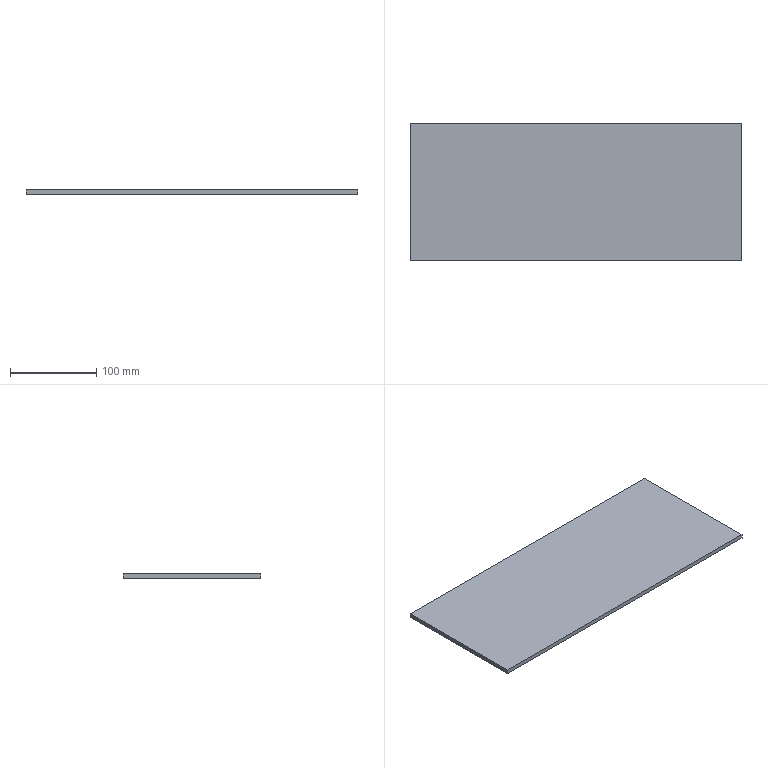Part | STEP file | FHD-021-014-03 acrylic | 1 solid | 6 faces | box 385 x 160 x 5 mm | volume 308000 mm3 | plane 6
STEP:
#1=CARTESIAN_POINT('',(0.,0.,0.));
#2=DIRECTION('',(0.,0.,1.));
#3=DIRECTION('',(1.,0.,0.));
#4=AXIS2_PLACEMENT_3D('',#1,#2,#3);
#5=CARTESIAN_POINT('',(-192.5,80.,5.));
#6=VERTEX_POINT('',#5);
#7=CARTESIAN_POINT('',(192.5,80.,5.));
#8=VERTEX_POINT('',#7);
#9=CARTESIAN_POINT('',(0.,80.,5.));
#10=DIRECTION('',(1.,0.,0.));
#11=VECTOR('',#10,1.);
#12=LINE('',#9,#11);
#13=CARTESIAN_POINT('',(0.,0.,5.));
#14=DIRECTION('',(0.,0.,-1.));
#15=DIRECTION('',(-1.,0.,0.));
#16=AXIS2_PLACEMENT_3D('',#13,#14,#15);
#17=PLANE('',#16);
#18=CARTESIAN_POINT('',(0.,80.));
#19=DIRECTION('',(-1.,0.));
#20=VECTOR('',#19,1.);
#21=LINE('',#18,#20);
#22=(GEOMETRIC_REPRESENTATION_CONTEXT(2)PARAMETRIC_REPRESENTATION_CONTEXT()REPRESENTATION_CONTEXT('',''));
#23=DEFINITIONAL_REPRESENTATION('',(#21),#22);
#24=PCURVE('',#17,#23);
#25=CARTESIAN_POINT('',(-192.5,80.,5.));
#26=DIRECTION('',(0.,-1.,0.));
#27=DIRECTION('',(0.,0.,-1.));
#28=AXIS2_PLACEMENT_3D('',#25,#26,#27);
#29=PLANE('',#28);
#30=CARTESIAN_POINT('',(0.,192.5));
#31=DIRECTION('',(0.,1.));
#32=VECTOR('',#31,1.);
#33=LINE('',#30,#32);
#34=(GEOMETRIC_REPRESENTATION_CONTEXT(2)PARAMETRIC_REPRESENTATION_CONTEXT()REPRESENTATION_CONTEXT('',''));
#35=DEFINITIONAL_REPRESENTATION('',(#33),#34);
#36=PCURVE('',#29,#35);
#37=SURFACE_CURVE('',#12,(#24,#36),.PCURVE_S1.);
#38=EDGE_CURVE('',#6,#8,#37,.T.);
#39=ORIENTED_EDGE('',*,*,#38,.F.);
#40=CARTESIAN_POINT('',(-192.5,-80.,5.));
#41=VERTEX_POINT('',#40);
#42=CARTESIAN_POINT('',(-192.5,0.,5.));
#43=DIRECTION('',(0.,1.,0.));
#44=VECTOR('',#43,1.);
#45=LINE('',#42,#44);
#46=CARTESIAN_POINT('',(192.5,0.));
#47=DIRECTION('',(0.,1.));
#48=VECTOR('',#47,1.);
#49=LINE('',#46,#48);
#50=(GEOMETRIC_REPRESENTATION_CONTEXT(2)PARAMETRIC_REPRESENTATION_CONTEXT()REPRESENTATION_CONTEXT('',''));
#51=DEFINITIONAL_REPRESENTATION('',(#49),#50);
#52=PCURVE('',#17,#51);
#53=CARTESIAN_POINT('',(-192.5,-80.,5.));
#54=DIRECTION('',(1.,0.,0.));
#55=DIRECTION('',(0.,0.,-1.));
#56=AXIS2_PLACEMENT_3D('',#53,#54,#55);
#57=PLANE('',#56);
#58=CARTESIAN_POINT('',(0.,80.));
#59=DIRECTION('',(0.,1.));
#60=VECTOR('',#59,1.);
#61=LINE('',#58,#60);
#62=(GEOMETRIC_REPRESENTATION_CONTEXT(2)PARAMETRIC_REPRESENTATION_CONTEXT()REPRESENTATION_CONTEXT('',''));
#63=DEFINITIONAL_REPRESENTATION('',(#61),#62);
#64=PCURVE('',#57,#63);
#65=SURFACE_CURVE('',#45,(#52,#64),.PCURVE_S1.);
#66=EDGE_CURVE('',#41,#6,#65,.T.);
#67=ORIENTED_EDGE('',*,*,#66,.F.);
#68=CARTESIAN_POINT('',(192.5,-80.,5.));
#69=VERTEX_POINT('',#68);
#70=CARTESIAN_POINT('',(0.,-80.,5.));
#71=DIRECTION('',(-1.,0.,0.));
#72=VECTOR('',#71,1.);
#73=LINE('',#70,#72);
#74=CARTESIAN_POINT('',(0.,-80.));
#75=DIRECTION('',(1.,0.));
#76=VECTOR('',#75,1.);
#77=LINE('',#74,#76);
#78=(GEOMETRIC_REPRESENTATION_CONTEXT(2)PARAMETRIC_REPRESENTATION_CONTEXT()REPRESENTATION_CONTEXT('',''));
#79=DEFINITIONAL_REPRESENTATION('',(#77),#78);
#80=PCURVE('',#17,#79);
#81=CARTESIAN_POINT('',(-192.5,-80.,5.));
#82=DIRECTION('',(0.,1.,0.));
#83=DIRECTION('',(0.,0.,1.));
#84=AXIS2_PLACEMENT_3D('',#81,#82,#83);
#85=PLANE('',#84);
#86=CARTESIAN_POINT('',(0.,192.5));
#87=DIRECTION('',(0.,-1.));
#88=VECTOR('',#87,1.);
#89=LINE('',#86,#88);
#90=(GEOMETRIC_REPRESENTATION_CONTEXT(2)PARAMETRIC_REPRESENTATION_CONTEXT()REPRESENTATION_CONTEXT('',''));
#91=DEFINITIONAL_REPRESENTATION('',(#89),#90);
#92=PCURVE('',#85,#91);
#93=SURFACE_CURVE('',#73,(#80,#92),.PCURVE_S1.);
#94=EDGE_CURVE('',#69,#41,#93,.T.);
#95=ORIENTED_EDGE('',*,*,#94,.F.);
#96=CARTESIAN_POINT('',(192.5,0.,5.));
#97=DIRECTION('',(0.,-1.,0.));
#98=VECTOR('',#97,1.);
#99=LINE('',#96,#98);
#100=CARTESIAN_POINT('',(-192.5,0.));
#101=DIRECTION('',(0.,-1.));
#102=VECTOR('',#101,1.);
#103=LINE('',#100,#102);
#104=(GEOMETRIC_REPRESENTATION_CONTEXT(2)PARAMETRIC_REPRESENTATION_CONTEXT()REPRESENTATION_CONTEXT('',''));
#105=DEFINITIONAL_REPRESENTATION('',(#103),#104);
#106=PCURVE('',#17,#105);
#107=CARTESIAN_POINT('',(192.5,-80.,5.));
#108=DIRECTION('',(-1.,0.,0.));
#109=DIRECTION('',(0.,0.,1.));
#110=AXIS2_PLACEMENT_3D('',#107,#108,#109);
#111=PLANE('',#110);
#112=CARTESIAN_POINT('',(0.,80.));
#113=DIRECTION('',(0.,-1.));
#114=VECTOR('',#113,1.);
#115=LINE('',#112,#114);
#116=(GEOMETRIC_REPRESENTATION_CONTEXT(2)PARAMETRIC_REPRESENTATION_CONTEXT()REPRESENTATION_CONTEXT('',''));
#117=DEFINITIONAL_REPRESENTATION('',(#115),#116);
#118=PCURVE('',#111,#117);
#119=SURFACE_CURVE('',#99,(#106,#118),.PCURVE_S1.);
#120=EDGE_CURVE('',#8,#69,#119,.T.);
#121=ORIENTED_EDGE('',*,*,#120,.F.);
#122=EDGE_LOOP('',(#39,#67,#95,#121));
#123=FACE_BOUND('',#122,.T.);
#124=ADVANCED_FACE('',(#123),#17,.F.);
#125=CARTESIAN_POINT('',(192.5,80.,0.));
#126=VERTEX_POINT('',#125);
#127=CARTESIAN_POINT('',(192.5,80.,5.));
#128=DIRECTION('',(0.,0.,-1.));
#129=VECTOR('',#128,1.);
#130=LINE('',#127,#129);
#131=CARTESIAN_POINT('',(0.,160.));
#132=DIRECTION('',(-1.,0.));
#133=VECTOR('',#132,1.);
#134=LINE('',#131,#133);
#135=(GEOMETRIC_REPRESENTATION_CONTEXT(2)PARAMETRIC_REPRESENTATION_CONTEXT()REPRESENTATION_CONTEXT('',''));
#136=DEFINITIONAL_REPRESENTATION('',(#134),#135);
#137=PCURVE('',#111,#136);
#138=CARTESIAN_POINT('',(0.,385.));
#139=DIRECTION('',(1.,0.));
#140=VECTOR('',#139,1.);
#141=LINE('',#138,#140);
#142=(GEOMETRIC_REPRESENTATION_CONTEXT(2)PARAMETRIC_REPRESENTATION_CONTEXT()REPRESENTATION_CONTEXT('',''));
#143=DEFINITIONAL_REPRESENTATION('',(#141),#142);
#144=PCURVE('',#29,#143);
#145=SURFACE_CURVE('',#130,(#137,#144),.PCURVE_S1.);
#146=EDGE_CURVE('',#8,#126,#145,.T.);
#147=ORIENTED_EDGE('',*,*,#146,.F.);
#148=ORIENTED_EDGE('',*,*,#120,.T.);
#149=CARTESIAN_POINT('',(192.5,-80.,0.));
#150=VERTEX_POINT('',#149);
#151=CARTESIAN_POINT('',(192.5,-80.,5.));
#152=DIRECTION('',(0.,0.,1.));
#153=VECTOR('',#152,1.);
#154=LINE('',#151,#153);
#155=CARTESIAN_POINT('',(0.,0.));
#156=DIRECTION('',(1.,0.));
#157=VECTOR('',#156,1.);
#158=LINE('',#155,#157);
#159=(GEOMETRIC_REPRESENTATION_CONTEXT(2)PARAMETRIC_REPRESENTATION_CONTEXT()REPRESENTATION_CONTEXT('',''));
#160=DEFINITIONAL_REPRESENTATION('',(#158),#159);
#161=PCURVE('',#111,#160);
#162=CARTESIAN_POINT('',(0.,385.));
#163=DIRECTION('',(1.,0.));
#164=VECTOR('',#163,1.);
#165=LINE('',#162,#164);
#166=(GEOMETRIC_REPRESENTATION_CONTEXT(2)PARAMETRIC_REPRESENTATION_CONTEXT()REPRESENTATION_CONTEXT('',''));
#167=DEFINITIONAL_REPRESENTATION('',(#165),#166);
#168=PCURVE('',#85,#167);
#169=SURFACE_CURVE('',#154,(#161,#168),.PCURVE_S1.);
#170=EDGE_CURVE('',#150,#69,#169,.T.);
#171=ORIENTED_EDGE('',*,*,#170,.F.);
#172=CARTESIAN_POINT('',(192.5,-80.,0.));
#173=DIRECTION('',(0.,-1.,0.));
#174=VECTOR('',#173,1.);
#175=LINE('',#172,#174);
#176=CARTESIAN_POINT('',(-5.,0.));
#177=DIRECTION('',(0.,-1.));
#178=VECTOR('',#177,1.);
#179=LINE('',#176,#178);
#180=(GEOMETRIC_REPRESENTATION_CONTEXT(2)PARAMETRIC_REPRESENTATION_CONTEXT()REPRESENTATION_CONTEXT('',''));
#181=DEFINITIONAL_REPRESENTATION('',(#179),#180);
#182=PCURVE('',#111,#181);
#183=CARTESIAN_POINT('',(0.,0.,0.));
#184=DIRECTION('',(0.,0.,-1.));
#185=DIRECTION('',(-1.,0.,0.));
#186=AXIS2_PLACEMENT_3D('',#183,#184,#185);
#187=PLANE('',#186);
#188=CARTESIAN_POINT('',(-192.5,-80.));
#189=DIRECTION('',(0.,-1.));
#190=VECTOR('',#189,1.);
#191=LINE('',#188,#190);
#192=(GEOMETRIC_REPRESENTATION_CONTEXT(2)PARAMETRIC_REPRESENTATION_CONTEXT()REPRESENTATION_CONTEXT('',''));
#193=DEFINITIONAL_REPRESENTATION('',(#191),#192);
#194=PCURVE('',#187,#193);
#195=SURFACE_CURVE('',#175,(#182,#194),.PCURVE_S1.);
#196=EDGE_CURVE('',#126,#150,#195,.T.);
#197=ORIENTED_EDGE('',*,*,#196,.F.);
#198=EDGE_LOOP('',(#147,#148,#171,#197));
#199=FACE_BOUND('',#198,.T.);
#200=ADVANCED_FACE('',(#199),#111,.F.);
#201=CARTESIAN_POINT('',(-192.5,80.,0.));
#202=VERTEX_POINT('',#201);
#203=CARTESIAN_POINT('',(-192.5,80.,5.));
#204=DIRECTION('',(0.,0.,-1.));
#205=VECTOR('',#204,1.);
#206=LINE('',#203,#205);
#207=CARTESIAN_POINT('',(0.,0.));
#208=DIRECTION('',(1.,0.));
#209=VECTOR('',#208,1.);
#210=LINE('',#207,#209);
#211=(GEOMETRIC_REPRESENTATION_CONTEXT(2)PARAMETRIC_REPRESENTATION_CONTEXT()REPRESENTATION_CONTEXT('',''));
#212=DEFINITIONAL_REPRESENTATION('',(#210),#211);
#213=PCURVE('',#29,#212);
#214=CARTESIAN_POINT('',(0.,160.));
#215=DIRECTION('',(1.,0.));
#216=VECTOR('',#215,1.);
#217=LINE('',#214,#216);
#218=(GEOMETRIC_REPRESENTATION_CONTEXT(2)PARAMETRIC_REPRESENTATION_CONTEXT()REPRESENTATION_CONTEXT('',''));
#219=DEFINITIONAL_REPRESENTATION('',(#217),#218);
#220=PCURVE('',#57,#219);
#221=SURFACE_CURVE('',#206,(#213,#220),.PCURVE_S1.);
#222=EDGE_CURVE('',#6,#202,#221,.T.);
#223=ORIENTED_EDGE('',*,*,#222,.F.);
#224=ORIENTED_EDGE('',*,*,#38,.T.);
#225=ORIENTED_EDGE('',*,*,#146,.T.);
#226=CARTESIAN_POINT('',(-192.5,80.,0.));
#227=DIRECTION('',(1.,0.,0.));
#228=VECTOR('',#227,1.);
#229=LINE('',#226,#228);
#230=CARTESIAN_POINT('',(5.,0.));
#231=DIRECTION('',(0.,1.));
#232=VECTOR('',#231,1.);
#233=LINE('',#230,#232);
#234=(GEOMETRIC_REPRESENTATION_CONTEXT(2)PARAMETRIC_REPRESENTATION_CONTEXT()REPRESENTATION_CONTEXT('',''));
#235=DEFINITIONAL_REPRESENTATION('',(#233),#234);
#236=PCURVE('',#29,#235);
#237=CARTESIAN_POINT('',(192.5,80.));
#238=DIRECTION('',(-1.,0.));
#239=VECTOR('',#238,1.);
#240=LINE('',#237,#239);
#241=(GEOMETRIC_REPRESENTATION_CONTEXT(2)PARAMETRIC_REPRESENTATION_CONTEXT()REPRESENTATION_CONTEXT('',''));
#242=DEFINITIONAL_REPRESENTATION('',(#240),#241);
#243=PCURVE('',#187,#242);
#244=SURFACE_CURVE('',#229,(#236,#243),.PCURVE_S1.);
#245=EDGE_CURVE('',#202,#126,#244,.T.);
#246=ORIENTED_EDGE('',*,*,#245,.F.);
#247=EDGE_LOOP('',(#223,#224,#225,#246));
#248=FACE_BOUND('',#247,.T.);
#249=ADVANCED_FACE('',(#248),#29,.F.);
#250=CARTESIAN_POINT('',(-192.5,-80.,0.));
#251=VERTEX_POINT('',#250);
#252=CARTESIAN_POINT('',(-192.5,-80.,5.));
#253=DIRECTION('',(0.,0.,-1.));
#254=VECTOR('',#253,1.);
#255=LINE('',#252,#254);
#256=CARTESIAN_POINT('',(0.,0.));
#257=DIRECTION('',(1.,0.));
#258=VECTOR('',#257,1.);
#259=LINE('',#256,#258);
#260=(GEOMETRIC_REPRESENTATION_CONTEXT(2)PARAMETRIC_REPRESENTATION_CONTEXT()REPRESENTATION_CONTEXT('',''));
#261=DEFINITIONAL_REPRESENTATION('',(#259),#260);
#262=PCURVE('',#57,#261);
#263=CARTESIAN_POINT('',(0.,0.));
#264=DIRECTION('',(-1.,0.));
#265=VECTOR('',#264,1.);
#266=LINE('',#263,#265);
#267=(GEOMETRIC_REPRESENTATION_CONTEXT(2)PARAMETRIC_REPRESENTATION_CONTEXT()REPRESENTATION_CONTEXT('',''));
#268=DEFINITIONAL_REPRESENTATION('',(#266),#267);
#269=PCURVE('',#85,#268);
#270=SURFACE_CURVE('',#255,(#262,#269),.PCURVE_S1.);
#271=EDGE_CURVE('',#41,#251,#270,.T.);
#272=ORIENTED_EDGE('',*,*,#271,.F.);
#273=ORIENTED_EDGE('',*,*,#66,.T.);
#274=ORIENTED_EDGE('',*,*,#222,.T.);
#275=CARTESIAN_POINT('',(-192.5,-80.,0.));
#276=DIRECTION('',(0.,1.,0.));
#277=VECTOR('',#276,1.);
#278=LINE('',#275,#277);
#279=CARTESIAN_POINT('',(5.,0.));
#280=DIRECTION('',(0.,1.));
#281=VECTOR('',#280,1.);
#282=LINE('',#279,#281);
#283=(GEOMETRIC_REPRESENTATION_CONTEXT(2)PARAMETRIC_REPRESENTATION_CONTEXT()REPRESENTATION_CONTEXT('',''));
#284=DEFINITIONAL_REPRESENTATION('',(#282),#283);
#285=PCURVE('',#57,#284);
#286=CARTESIAN_POINT('',(192.5,-80.));
#287=DIRECTION('',(0.,1.));
#288=VECTOR('',#287,1.);
#289=LINE('',#286,#288);
#290=(GEOMETRIC_REPRESENTATION_CONTEXT(2)PARAMETRIC_REPRESENTATION_CONTEXT()REPRESENTATION_CONTEXT('',''));
#291=DEFINITIONAL_REPRESENTATION('',(#289),#290);
#292=PCURVE('',#187,#291);
#293=SURFACE_CURVE('',#278,(#285,#292),.PCURVE_S1.);
#294=EDGE_CURVE('',#251,#202,#293,.T.);
#295=ORIENTED_EDGE('',*,*,#294,.F.);
#296=EDGE_LOOP('',(#272,#273,#274,#295));
#297=FACE_BOUND('',#296,.T.);
#298=ADVANCED_FACE('',(#297),#57,.F.);
#299=ORIENTED_EDGE('',*,*,#170,.T.);
#300=ORIENTED_EDGE('',*,*,#94,.T.);
#301=ORIENTED_EDGE('',*,*,#271,.T.);
#302=CARTESIAN_POINT('',(-192.5,-80.,0.));
#303=DIRECTION('',(-1.,0.,0.));
#304=VECTOR('',#303,1.);
#305=LINE('',#302,#304);
#306=CARTESIAN_POINT('',(-5.,0.));
#307=DIRECTION('',(0.,-1.));
#308=VECTOR('',#307,1.);
#309=LINE('',#306,#308);
#310=(GEOMETRIC_REPRESENTATION_CONTEXT(2)PARAMETRIC_REPRESENTATION_CONTEXT()REPRESENTATION_CONTEXT('',''));
#311=DEFINITIONAL_REPRESENTATION('',(#309),#310);
#312=PCURVE('',#85,#311);
#313=CARTESIAN_POINT('',(192.5,-80.));
#314=DIRECTION('',(1.,0.));
#315=VECTOR('',#314,1.);
#316=LINE('',#313,#315);
#317=(GEOMETRIC_REPRESENTATION_CONTEXT(2)PARAMETRIC_REPRESENTATION_CONTEXT()REPRESENTATION_CONTEXT('',''));
#318=DEFINITIONAL_REPRESENTATION('',(#316),#317);
#319=PCURVE('',#187,#318);
#320=SURFACE_CURVE('',#305,(#312,#319),.PCURVE_S1.);
#321=EDGE_CURVE('',#150,#251,#320,.T.);
#322=ORIENTED_EDGE('',*,*,#321,.F.);
#323=EDGE_LOOP('',(#299,#300,#301,#322));
#324=FACE_BOUND('',#323,.T.);
#325=ADVANCED_FACE('',(#324),#85,.F.);
#326=ORIENTED_EDGE('',*,*,#294,.T.);
#327=ORIENTED_EDGE('',*,*,#245,.T.);
#328=ORIENTED_EDGE('',*,*,#196,.T.);
#329=ORIENTED_EDGE('',*,*,#321,.T.);
#330=EDGE_LOOP('',(#326,#327,#328,#329));
#331=FACE_BOUND('',#330,.T.);
#332=ADVANCED_FACE('',(#331),#187,.T.);
#333=CLOSED_SHELL('',(#124,#200,#249,#298,#325,#332));
#334=MANIFOLD_SOLID_BREP('',#333);
#335=(LENGTH_UNIT()NAMED_UNIT(*)SI_UNIT(.MILLI.,.METRE.));
#336=UNCERTAINTY_MEASURE_WITH_UNIT(LENGTH_MEASURE(0.0000001),#335,'','');
#337=(NAMED_UNIT(*)PLANE_ANGLE_UNIT()SI_UNIT($,.RADIAN.));
#338=(NAMED_UNIT(*)SI_UNIT($,.STERADIAN.)SOLID_ANGLE_UNIT());
#339=(GEOMETRIC_REPRESENTATION_CONTEXT(3)GLOBAL_UNCERTAINTY_ASSIGNED_CONTEXT((#336))GLOBAL_UNIT_ASSIGNED_CONTEXT((#335,#337,#338))REPRESENTATION_CONTEXT('',''));
#340=ADVANCED_BREP_SHAPE_REPRESENTATION('',(#4,#334),#339);